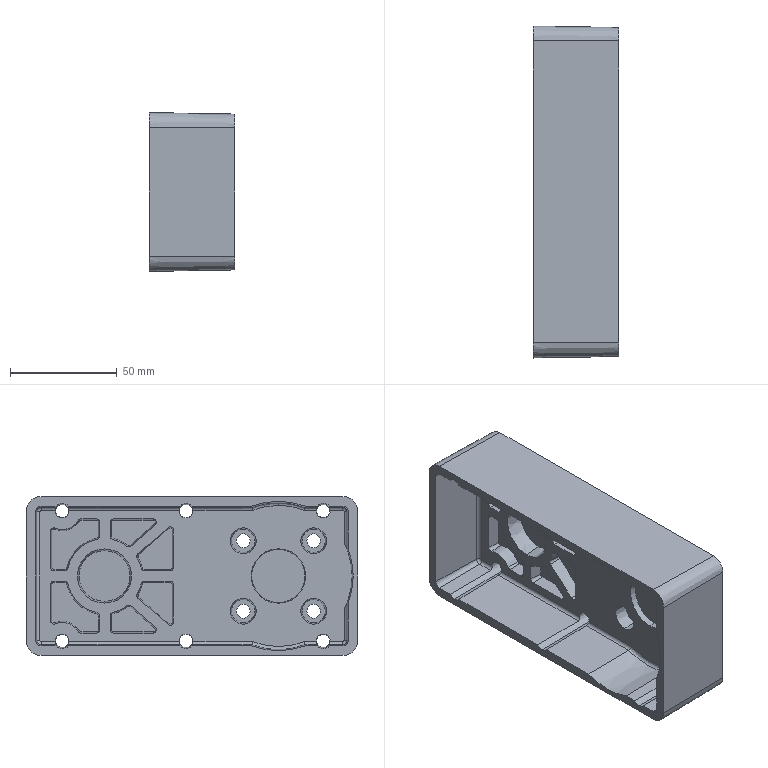Part | SolidWorks | features BaseBody 1 | 1 solid | 176 faces | box 40 x 155.42 x 74.42 mm | volume 165846 mm3 | cone 90 | plane 58 | cylinder 21 | spline 7 | commonest cylinder face diameters 3 x13 6.4 x8